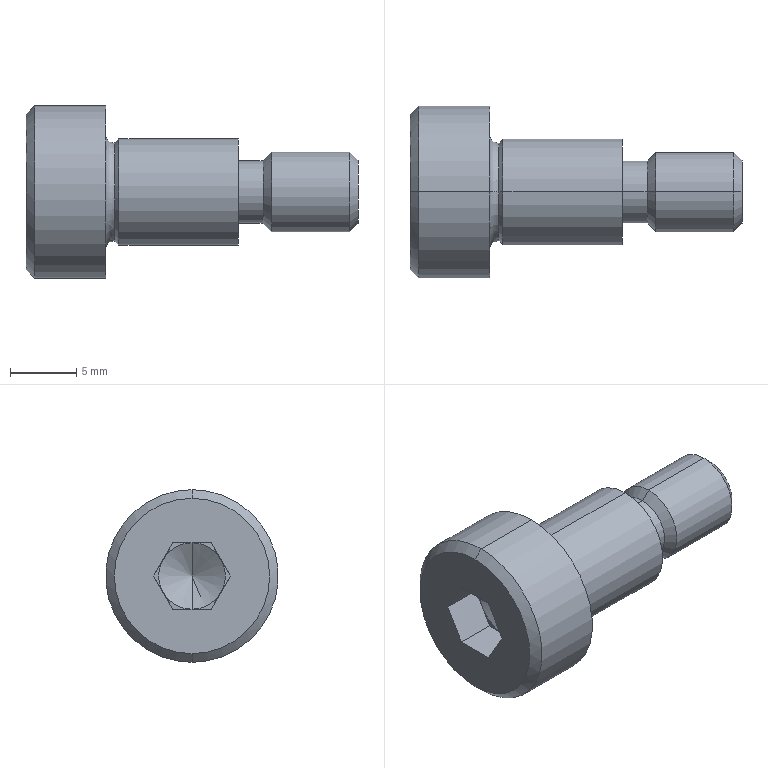Part | STEP file | 11-MSB8_1011_MSB8-10 | 1 solid | 38 faces | box 25 x 13 x 13 mm | volume 1439 mm3 | plane 16 | cone 10 | cylinder 8 | torus 4 | commonest cylinder face diameters 4.7 x2 6 x2 8 x2 13 x2
STEP:
#1=CARTESIAN_POINT('',(0.,0.,4.35));
#2=VERTEX_POINT('',#1);
#3=CARTESIAN_POINT('',(0.6306,0.,3.696));
#4=VERTEX_POINT('',#3);
#5=CARTESIAN_POINT('',(0.6306,0.,4.327));
#6=DIRECTION('',(0.,-1.,0.));
#7=DIRECTION('',(0.,0.,-1.));
#8=AXIS2_PLACEMENT_3D('',#5,#6,#7);
#9=CIRCLE('',#8,0.631);
#10=EDGE_CURVE('',#2,#4,#9,.T.);
#11=ORIENTED_EDGE('',*,*,#10,.T.);
#12=CARTESIAN_POINT('',(0.6306,0.,-3.696));
#13=VERTEX_POINT('',#12);
#14=CARTESIAN_POINT('',(0.6306,0.,0.));
#15=DIRECTION('',(-1.,0.,0.));
#16=DIRECTION('',(0.,0.,1.));
#17=AXIS2_PLACEMENT_3D('',#14,#15,#16);
#18=CIRCLE('',#17,3.696);
#19=EDGE_CURVE('',#4,#13,#18,.T.);
#20=ORIENTED_EDGE('',*,*,#19,.T.);
#21=CARTESIAN_POINT('',(0.,0.,-4.35));
#22=VERTEX_POINT('',#21);
#23=CARTESIAN_POINT('',(0.6306,0.,-4.327));
#24=DIRECTION('',(0.,1.,0.));
#25=DIRECTION('',(0.,0.,1.));
#26=AXIS2_PLACEMENT_3D('',#23,#24,#25);
#27=CIRCLE('',#26,0.631);
#28=EDGE_CURVE('',#22,#13,#27,.T.);
#29=ORIENTED_EDGE('',*,*,#28,.F.);
#30=CARTESIAN_POINT('',(0.,0.,0.));
#31=DIRECTION('',(-1.,0.,0.));
#32=DIRECTION('',(0.,0.,1.));
#33=AXIS2_PLACEMENT_3D('',#30,#31,#32);
#34=CIRCLE('',#33,4.35);
#35=EDGE_CURVE('',#2,#22,#34,.T.);
#36=ORIENTED_EDGE('',*,*,#35,.F.);
#37=EDGE_LOOP('',(#11,#20,#29,#36));
#38=FACE_OUTER_BOUND('',#37,.T.);
#39=CARTESIAN_POINT('',(0.6306,0.,0.));
#40=DIRECTION('',(-1.,0.,0.));
#41=DIRECTION('',(0.,0.,1.));
#42=AXIS2_PLACEMENT_3D('',#39,#40,#41);
#43=TOROIDAL_SURFACE('',#42,4.327,0.631);
#44=ADVANCED_FACE('',(#38),#43,.F.);
#45=ORIENTED_EDGE('',*,*,#28,.T.);
#46=CARTESIAN_POINT('',(0.6306,0.,0.));
#47=DIRECTION('',(-1.,0.,0.));
#48=DIRECTION('',(0.,0.,1.));
#49=AXIS2_PLACEMENT_3D('',#46,#47,#48);
#50=CIRCLE('',#49,3.696);
#51=EDGE_CURVE('',#13,#4,#50,.T.);
#52=ORIENTED_EDGE('',*,*,#51,.T.);
#53=ORIENTED_EDGE('',*,*,#10,.F.);
#54=CARTESIAN_POINT('',(0.,0.,0.));
#55=DIRECTION('',(-1.,0.,0.));
#56=DIRECTION('',(0.,0.,1.));
#57=AXIS2_PLACEMENT_3D('',#54,#55,#56);
#58=CIRCLE('',#57,4.35);
#59=EDGE_CURVE('',#22,#2,#58,.T.);
#60=ORIENTED_EDGE('',*,*,#59,.F.);
#61=EDGE_LOOP('',(#45,#52,#53,#60));
#62=FACE_OUTER_BOUND('',#61,.T.);
#63=CARTESIAN_POINT('',(0.6306,0.,0.));
#64=DIRECTION('',(-1.,0.,0.));
#65=DIRECTION('',(0.,0.,1.));
#66=AXIS2_PLACEMENT_3D('',#63,#64,#65);
#67=TOROIDAL_SURFACE('',#66,4.327,0.631);
#68=ADVANCED_FACE('',(#62),#67,.F.);
#69=CARTESIAN_POINT('',(-1.557,0.,0.));
#70=VERTEX_POINT('',#69);
#71=CARTESIAN_POINT('',(-3.,0.,2.5));
#72=VERTEX_POINT('',#71);
#73=CARTESIAN_POINT('',(-3.,0.,2.5));
#74=DIRECTION('',(-0.5,0.,0.866));
#75=VECTOR('',#74,1000.);
#76=LINE('',#73,#75);
#77=EDGE_CURVE('',#70,#72,#76,.T.);
#78=ORIENTED_EDGE('',*,*,#77,.F.);
#79=CARTESIAN_POINT('',(-3.,0.,-2.5));
#80=VERTEX_POINT('',#79);
#81=CARTESIAN_POINT('',(-3.,0.,-2.5));
#82=DIRECTION('',(-0.5,0.,-0.866));
#83=VECTOR('',#82,1000.);
#84=LINE('',#81,#83);
#85=EDGE_CURVE('',#70,#80,#84,.T.);
#86=ORIENTED_EDGE('',*,*,#85,.T.);
#87=CARTESIAN_POINT('',(-3.,-2.165,-1.25));
#88=VERTEX_POINT('',#87);
#89=CARTESIAN_POINT('',(-3.,0.,0.));
#90=DIRECTION('',(-1.,0.,0.));
#91=DIRECTION('',(0.,0.,1.));
#92=AXIS2_PLACEMENT_3D('',#89,#90,#91);
#93=CIRCLE('',#92,2.5);
#94=EDGE_CURVE('',#80,#88,#93,.T.);
#95=ORIENTED_EDGE('',*,*,#94,.T.);
#96=CARTESIAN_POINT('',(-3.,-2.165,1.25));
#97=VERTEX_POINT('',#96);
#98=CARTESIAN_POINT('',(-3.,0.,0.));
#99=DIRECTION('',(-1.,0.,0.));
#100=DIRECTION('',(0.,0.,1.));
#101=AXIS2_PLACEMENT_3D('',#98,#99,#100);
#102=CIRCLE('',#101,2.5);
#103=EDGE_CURVE('',#88,#97,#102,.T.);
#104=ORIENTED_EDGE('',*,*,#103,.T.);
#105=CARTESIAN_POINT('',(-3.,0.,0.));
#106=DIRECTION('',(-1.,0.,0.));
#107=DIRECTION('',(0.,0.,1.));
#108=AXIS2_PLACEMENT_3D('',#105,#106,#107);
#109=CIRCLE('',#108,2.5);
#110=EDGE_CURVE('',#97,#72,#109,.T.);
#111=ORIENTED_EDGE('',*,*,#110,.T.);
#112=EDGE_LOOP('',(#78,#86,#95,#104,#111));
#113=FACE_OUTER_BOUND('',#112,.T.);
#114=CARTESIAN_POINT('',(-3.,0.,0.));
#115=DIRECTION('',(-1.,0.,0.));
#116=DIRECTION('',(0.,0.,1.));
#117=AXIS2_PLACEMENT_3D('',#114,#115,#116);
#118=CONICAL_SURFACE('',#117,2.5,1.047);
#119=ADVANCED_FACE('',(#113),#118,.F.);
#120=CARTESIAN_POINT('',(-6.,0.,5.85));
#121=VERTEX_POINT('',#120);
#122=CARTESIAN_POINT('',(-6.,0.,-5.85));
#123=VERTEX_POINT('',#122);
#124=CARTESIAN_POINT('',(-6.,0.,0.));
#125=DIRECTION('',(-1.,0.,0.));
#126=DIRECTION('',(0.,0.,1.));
#127=AXIS2_PLACEMENT_3D('',#124,#125,#126);
#128=CIRCLE('',#127,5.85);
#129=EDGE_CURVE('',#121,#123,#128,.T.);
#130=ORIENTED_EDGE('',*,*,#129,.F.);
#131=CARTESIAN_POINT('',(-5.35,0.,6.5));
#132=VERTEX_POINT('',#131);
#133=CARTESIAN_POINT('',(-5.35,0.,6.5));
#134=DIRECTION('',(0.7071,0.,0.7071));
#135=VECTOR('',#134,1000.);
#136=LINE('',#133,#135);
#137=EDGE_CURVE('',#121,#132,#136,.T.);
#138=ORIENTED_EDGE('',*,*,#137,.T.);
#139=CARTESIAN_POINT('',(-5.35,0.,-6.5));
#140=VERTEX_POINT('',#139);
#141=CARTESIAN_POINT('',(-5.35,0.,0.));
#142=DIRECTION('',(-1.,0.,0.));
#143=DIRECTION('',(0.,0.,1.));
#144=AXIS2_PLACEMENT_3D('',#141,#142,#143);
#145=CIRCLE('',#144,6.5);
#146=EDGE_CURVE('',#132,#140,#145,.T.);
#147=ORIENTED_EDGE('',*,*,#146,.T.);
#148=CARTESIAN_POINT('',(-5.35,0.,-6.5));
#149=DIRECTION('',(0.7071,0.,-0.7071));
#150=VECTOR('',#149,1000.);
#151=LINE('',#148,#150);
#152=EDGE_CURVE('',#123,#140,#151,.T.);
#153=ORIENTED_EDGE('',*,*,#152,.F.);
#154=EDGE_LOOP('',(#130,#138,#147,#153));
#155=FACE_OUTER_BOUND('',#154,.T.);
#156=CARTESIAN_POINT('',(-5.35,0.,0.));
#157=DIRECTION('',(1.,0.,0.));
#158=DIRECTION('',(0.,0.,-1.));
#159=AXIS2_PLACEMENT_3D('',#156,#157,#158);
#160=CONICAL_SURFACE('',#159,6.5,0.7854);
#161=ADVANCED_FACE('',(#155),#160,.T.);
#162=CARTESIAN_POINT('',(0.,0.,6.5));
#163=VERTEX_POINT('',#162);
#164=CARTESIAN_POINT('',(0.,0.,-6.5));
#165=VERTEX_POINT('',#164);
#166=CARTESIAN_POINT('',(0.,0.,0.));
#167=DIRECTION('',(-1.,0.,0.));
#168=DIRECTION('',(0.,0.,1.));
#169=AXIS2_PLACEMENT_3D('',#166,#167,#168);
#170=CIRCLE('',#169,6.5);
#171=EDGE_CURVE('',#163,#165,#170,.T.);
#172=ORIENTED_EDGE('',*,*,#171,.T.);
#173=CARTESIAN_POINT('',(19.,0.,-6.5));
#174=DIRECTION('',(-1.,0.,0.));
#175=VECTOR('',#174,1000.);
#176=LINE('',#173,#175);
#177=EDGE_CURVE('',#165,#140,#176,.T.);
#178=ORIENTED_EDGE('',*,*,#177,.T.);
#179=ORIENTED_EDGE('',*,*,#146,.F.);
#180=CARTESIAN_POINT('',(19.,0.,6.5));
#181=DIRECTION('',(-1.,0.,0.));
#182=VECTOR('',#181,1000.);
#183=LINE('',#180,#182);
#184=EDGE_CURVE('',#163,#132,#183,.T.);
#185=ORIENTED_EDGE('',*,*,#184,.F.);
#186=EDGE_LOOP('',(#172,#178,#179,#185));
#187=FACE_OUTER_BOUND('',#186,.T.);
#188=CARTESIAN_POINT('',(19.,0.,0.));
#189=DIRECTION('',(-1.,0.,0.));
#190=DIRECTION('',(0.,0.,1.));
#191=AXIS2_PLACEMENT_3D('',#188,#189,#190);
#192=CYLINDRICAL_SURFACE('',#191,6.5);
#193=ADVANCED_FACE('',(#187),#192,.T.);
#194=ORIENTED_EDGE('',*,*,#51,.F.);
#195=CARTESIAN_POINT('',(0.7,0.,-3.7));
#196=VERTEX_POINT('',#195);
#197=CARTESIAN_POINT('',(0.6306,0.,-4.327));
#198=DIRECTION('',(0.,1.,0.));
#199=DIRECTION('',(0.,0.,1.));
#200=AXIS2_PLACEMENT_3D('',#197,#198,#199);
#201=CIRCLE('',#200,0.631);
#202=EDGE_CURVE('',#13,#196,#201,.T.);
#203=ORIENTED_EDGE('',*,*,#202,.T.);
#204=CARTESIAN_POINT('',(0.7,0.,3.7));
#205=VERTEX_POINT('',#204);
#206=CARTESIAN_POINT('',(0.7,0.,0.));
#207=DIRECTION('',(-1.,0.,0.));
#208=DIRECTION('',(0.,0.,1.));
#209=AXIS2_PLACEMENT_3D('',#206,#207,#208);
#210=CIRCLE('',#209,3.7);
#211=EDGE_CURVE('',#196,#205,#210,.T.);
#212=ORIENTED_EDGE('',*,*,#211,.T.);
#213=CARTESIAN_POINT('',(0.6306,0.,4.327));
#214=DIRECTION('',(0.,-1.,0.));
#215=DIRECTION('',(0.,0.,-1.));
#216=AXIS2_PLACEMENT_3D('',#213,#214,#215);
#217=CIRCLE('',#216,0.631);
#218=EDGE_CURVE('',#4,#205,#217,.T.);
#219=ORIENTED_EDGE('',*,*,#218,.F.);
#220=EDGE_LOOP('',(#194,#203,#212,#219));
#221=FACE_OUTER_BOUND('',#220,.T.);
#222=CARTESIAN_POINT('',(0.6306,0.,0.));
#223=DIRECTION('',(-1.,0.,0.));
#224=DIRECTION('',(0.,0.,1.));
#225=AXIS2_PLACEMENT_3D('',#222,#223,#224);
#226=TOROIDAL_SURFACE('',#225,4.327,0.631);
#227=ADVANCED_FACE('',(#221),#226,.F.);
#228=CARTESIAN_POINT('',(0.7,0.,0.));
#229=DIRECTION('',(-1.,0.,0.));
#230=DIRECTION('',(0.,0.,1.));
#231=AXIS2_PLACEMENT_3D('',#228,#229,#230);
#232=CIRCLE('',#231,3.7);
#233=EDGE_CURVE('',#205,#196,#232,.T.);
#234=ORIENTED_EDGE('',*,*,#233,.F.);
#235=CARTESIAN_POINT('',(1.,0.,4.));
#236=VERTEX_POINT('',#235);
#237=CARTESIAN_POINT('',(1.,0.,4.));
#238=DIRECTION('',(0.7071,0.,0.7071));
#239=VECTOR('',#238,1000.);
#240=LINE('',#237,#239);
#241=EDGE_CURVE('',#205,#236,#240,.T.);
#242=ORIENTED_EDGE('',*,*,#241,.T.);
#243=CARTESIAN_POINT('',(1.,0.,-4.));
#244=VERTEX_POINT('',#243);
#245=CARTESIAN_POINT('',(1.,0.,0.));
#246=DIRECTION('',(-1.,0.,0.));
#247=DIRECTION('',(0.,0.,1.));
#248=AXIS2_PLACEMENT_3D('',#245,#246,#247);
#249=CIRCLE('',#248,4.);
#250=EDGE_CURVE('',#236,#244,#249,.T.);
#251=ORIENTED_EDGE('',*,*,#250,.T.);
#252=CARTESIAN_POINT('',(1.,0.,-4.));
#253=DIRECTION('',(0.7071,0.,-0.7071));
#254=VECTOR('',#253,1000.);
#255=LINE('',#252,#254);
#256=EDGE_CURVE('',#196,#244,#255,.T.);
#257=ORIENTED_EDGE('',*,*,#256,.F.);
#258=EDGE_LOOP('',(#234,#242,#251,#257));
#259=FACE_OUTER_BOUND('',#258,.T.);
#260=CARTESIAN_POINT('',(1.,0.,0.));
#261=DIRECTION('',(1.,0.,0.));
#262=DIRECTION('',(0.,0.,-1.));
#263=AXIS2_PLACEMENT_3D('',#260,#261,#262);
#264=CONICAL_SURFACE('',#263,4.,0.7854);
#265=ADVANCED_FACE('',(#259),#264,.T.);
#266=CARTESIAN_POINT('',(10.,0.,4.));
#267=VERTEX_POINT('',#266);
#268=CARTESIAN_POINT('',(10.,0.,-4.));
#269=VERTEX_POINT('',#268);
#270=CARTESIAN_POINT('',(10.,0.,0.));
#271=DIRECTION('',(-1.,0.,0.));
#272=DIRECTION('',(0.,0.,1.));
#273=AXIS2_PLACEMENT_3D('',#270,#271,#272);
#274=CIRCLE('',#273,4.);
#275=EDGE_CURVE('',#267,#269,#274,.T.);
#276=ORIENTED_EDGE('',*,*,#275,.T.);
#277=CARTESIAN_POINT('',(19.,0.,-4.));
#278=DIRECTION('',(-1.,0.,0.));
#279=VECTOR('',#278,1000.);
#280=LINE('',#277,#279);
#281=EDGE_CURVE('',#269,#244,#280,.T.);
#282=ORIENTED_EDGE('',*,*,#281,.T.);
#283=ORIENTED_EDGE('',*,*,#250,.F.);
#284=CARTESIAN_POINT('',(19.,0.,4.));
#285=DIRECTION('',(-1.,0.,0.));
#286=VECTOR('',#285,1000.);
#287=LINE('',#284,#286);
#288=EDGE_CURVE('',#267,#236,#287,.T.);
#289=ORIENTED_EDGE('',*,*,#288,.F.);
#290=EDGE_LOOP('',(#276,#282,#283,#289));
#291=FACE_OUTER_BOUND('',#290,.T.);
#292=CARTESIAN_POINT('',(19.,0.,0.));
#293=DIRECTION('',(-1.,0.,0.));
#294=DIRECTION('',(0.,0.,1.));
#295=AXIS2_PLACEMENT_3D('',#292,#293,#294);
#296=CYLINDRICAL_SURFACE('',#295,4.);
#297=ADVANCED_FACE('',(#291),#296,.T.);
#298=CARTESIAN_POINT('',(11.85,0.,2.35));
#299=VERTEX_POINT('',#298);
#300=CARTESIAN_POINT('',(11.85,0.,-2.35));
#301=VERTEX_POINT('',#300);
#302=CARTESIAN_POINT('',(11.85,0.,0.));
#303=DIRECTION('',(-1.,0.,0.));
#304=DIRECTION('',(0.,0.,1.));
#305=AXIS2_PLACEMENT_3D('',#302,#303,#304);
#306=CIRCLE('',#305,2.35);
#307=EDGE_CURVE('',#299,#301,#306,.T.);
#308=ORIENTED_EDGE('',*,*,#307,.T.);
#309=CARTESIAN_POINT('',(10.,0.,-2.35));
#310=VERTEX_POINT('',#309);
#311=CARTESIAN_POINT('',(19.,0.,-2.35));
#312=DIRECTION('',(-1.,0.,0.));
#313=VECTOR('',#312,1000.);
#314=LINE('',#311,#313);
#315=EDGE_CURVE('',#301,#310,#314,.T.);
#316=ORIENTED_EDGE('',*,*,#315,.T.);
#317=CARTESIAN_POINT('',(10.,0.,2.35));
#318=VERTEX_POINT('',#317);
#319=CARTESIAN_POINT('',(10.,0.,0.));
#320=DIRECTION('',(-1.,0.,0.));
#321=DIRECTION('',(0.,0.,1.));
#322=AXIS2_PLACEMENT_3D('',#319,#320,#321);
#323=CIRCLE('',#322,2.35);
#324=EDGE_CURVE('',#318,#310,#323,.T.);
#325=ORIENTED_EDGE('',*,*,#324,.F.);
#326=CARTESIAN_POINT('',(19.,0.,2.35));
#327=DIRECTION('',(-1.,0.,0.));
#328=VECTOR('',#327,1000.);
#329=LINE('',#326,#328);
#330=EDGE_CURVE('',#299,#318,#329,.T.);
#331=ORIENTED_EDGE('',*,*,#330,.F.);
#332=EDGE_LOOP('',(#308,#316,#325,#331));
#333=FACE_OUTER_BOUND('',#332,.T.);
#334=CARTESIAN_POINT('',(19.,0.,0.));
#335=DIRECTION('',(-1.,0.,0.));
#336=DIRECTION('',(0.,0.,1.));
#337=AXIS2_PLACEMENT_3D('',#334,#335,#336);
#338=CYLINDRICAL_SURFACE('',#337,2.35);
#339=ADVANCED_FACE('',(#333),#338,.T.);
#340=ORIENTED_EDGE('',*,*,#307,.F.);
#341=CARTESIAN_POINT('',(12.5,0.,3.));
#342=VERTEX_POINT('',#341);
#343=CARTESIAN_POINT('',(12.5,0.,3.));
#344=DIRECTION('',(0.7071,0.,0.7071));
#345=VECTOR('',#344,1000.);
#346=LINE('',#343,#345);
#347=EDGE_CURVE('',#299,#342,#346,.T.);
#348=ORIENTED_EDGE('',*,*,#347,.T.);
#349=CARTESIAN_POINT('',(12.5,0.,-3.));
#350=VERTEX_POINT('',#349);
#351=CARTESIAN_POINT('',(12.5,0.,0.));
#352=DIRECTION('',(-1.,0.,0.));
#353=DIRECTION('',(0.,0.,1.));
#354=AXIS2_PLACEMENT_3D('',#351,#352,#353);
#355=CIRCLE('',#354,3.);
#356=EDGE_CURVE('',#342,#350,#355,.T.);
#357=ORIENTED_EDGE('',*,*,#356,.T.);
#358=CARTESIAN_POINT('',(12.5,0.,-3.));
#359=DIRECTION('',(0.7071,0.,-0.7071));
#360=VECTOR('',#359,1000.);
#361=LINE('',#358,#360);
#362=EDGE_CURVE('',#301,#350,#361,.T.);
#363=ORIENTED_EDGE('',*,*,#362,.F.);
#364=EDGE_LOOP('',(#340,#348,#357,#363));
#365=FACE_OUTER_BOUND('',#364,.T.);
#366=CARTESIAN_POINT('',(12.5,0.,0.));
#367=DIRECTION('',(1.,0.,0.));
#368=DIRECTION('',(0.,0.,-1.));
#369=AXIS2_PLACEMENT_3D('',#366,#367,#368);
#370=CONICAL_SURFACE('',#369,3.,0.7854);
#371=ADVANCED_FACE('',(#365),#370,.T.);
#372=CARTESIAN_POINT('',(18.387,0.,3.));
#373=VERTEX_POINT('',#372);
#374=CARTESIAN_POINT('',(18.387,0.,-3.));
#375=VERTEX_POINT('',#374);
#376=CARTESIAN_POINT('',(18.387,0.,0.));
#377=DIRECTION('',(-1.,0.,0.));
#378=DIRECTION('',(0.,0.,1.));
#379=AXIS2_PLACEMENT_3D('',#376,#377,#378);
#380=CIRCLE('',#379,3.);
#381=EDGE_CURVE('',#373,#375,#380,.T.);
#382=ORIENTED_EDGE('',*,*,#381,.T.);
#383=CARTESIAN_POINT('',(19.,0.,-3.));
#384=DIRECTION('',(-1.,0.,0.));
#385=VECTOR('',#384,1000.);
#386=LINE('',#383,#385);
#387=EDGE_CURVE('',#375,#350,#386,.T.);
#388=ORIENTED_EDGE('',*,*,#387,.T.);
#389=ORIENTED_EDGE('',*,*,#356,.F.);
#390=CARTESIAN_POINT('',(19.,0.,3.));
#391=DIRECTION('',(-1.,0.,0.));
#392=VECTOR('',#391,1000.);
#393=LINE('',#390,#392);
#394=EDGE_CURVE('',#373,#342,#393,.T.);
#395=ORIENTED_EDGE('',*,*,#394,.F.);
#396=EDGE_LOOP('',(#382,#388,#389,#395));
#397=FACE_OUTER_BOUND('',#396,.T.);
#398=CARTESIAN_POINT('',(19.,0.,0.));
#399=DIRECTION('',(-1.,0.,0.));
#400=DIRECTION('',(0.,0.,1.));
#401=AXIS2_PLACEMENT_3D('',#398,#399,#400);
#402=CYLINDRICAL_SURFACE('',#401,3.);
#403=ADVANCED_FACE('',(#397),#402,.T.);
#404=CARTESIAN_POINT('',(19.,0.,2.386));
#405=VERTEX_POINT('',#404);
#406=CARTESIAN_POINT('',(19.,0.,-2.386));
#407=VERTEX_POINT('',#406);
#408=CARTESIAN_POINT('',(19.,0.,0.));
#409=DIRECTION('',(-1.,0.,0.));
#410=DIRECTION('',(0.,0.,1.));
#411=AXIS2_PLACEMENT_3D('',#408,#409,#410);
#412=CIRCLE('',#411,2.386);
#413=EDGE_CURVE('',#405,#407,#412,.T.);
#414=ORIENTED_EDGE('',*,*,#413,.T.);
#415=CARTESIAN_POINT('',(19.,0.,-2.386));
#416=DIRECTION('',(-0.7071,0.,-0.7071));
#417=VECTOR('',#416,1000.);
#418=LINE('',#415,#417);
#419=EDGE_CURVE('',#407,#375,#418,.T.);
#420=ORIENTED_EDGE('',*,*,#419,.T.);
#421=ORIENTED_EDGE('',*,*,#381,.F.);
#422=CARTESIAN_POINT('',(19.,0.,2.386));
#423=DIRECTION('',(-0.7071,0.,0.7071));
#424=VECTOR('',#423,1000.);
#425=LINE('',#422,#424);
#426=EDGE_CURVE('',#405,#373,#425,.T.);
#427=ORIENTED_EDGE('',*,*,#426,.F.);
#428=EDGE_LOOP('',(#414,#420,#421,#427));
#429=FACE_OUTER_BOUND('',#428,.T.);
#430=CARTESIAN_POINT('',(19.,0.,0.));
#431=DIRECTION('',(-1.,0.,0.));
#432=DIRECTION('',(0.,0.,1.));
#433=AXIS2_PLACEMENT_3D('',#430,#431,#432);
#434=CONICAL_SURFACE('',#433,2.386,0.7854);
#435=ADVANCED_FACE('',(#429),#434,.T.);
#436=CARTESIAN_POINT('',(-6.,0.,0.));
#437=DIRECTION('',(-1.,0.,0.));
#438=DIRECTION('',(0.,0.,1.));
#439=AXIS2_PLACEMENT_3D('',#436,#437,#438);
#440=CIRCLE('',#439,5.85);
#441=EDGE_CURVE('',#123,#121,#440,.T.);
#442=ORIENTED_EDGE('',*,*,#441,.T.);
#443=ORIENTED_EDGE('',*,*,#129,.T.);
#444=EDGE_LOOP('',(#442,#443));
#445=FACE_OUTER_BOUND('',#444,.T.);
#446=CARTESIAN_POINT('',(-6.,-1.443,2.5));
#447=VERTEX_POINT('',#446);
#448=CARTESIAN_POINT('',(-6.,-2.887,0.));
#449=VERTEX_POINT('',#448);
#450=CARTESIAN_POINT('',(-6.,-1.443,2.5));
#451=DIRECTION('',(0.,-0.5,-0.866));
#452=VECTOR('',#451,1000.);
#453=LINE('',#450,#452);
#454=EDGE_CURVE('',#447,#449,#453,.T.);
#455=ORIENTED_EDGE('',*,*,#454,.T.);
#456=CARTESIAN_POINT('',(-6.,-1.443,-2.5));
#457=VERTEX_POINT('',#456);
#458=CARTESIAN_POINT('',(-6.,-2.887,0.));
#459=DIRECTION('',(0.,0.5,-0.866));
#460=VECTOR('',#459,1000.);
#461=LINE('',#458,#460);
#462=EDGE_CURVE('',#449,#457,#461,.T.);
#463=ORIENTED_EDGE('',*,*,#462,.T.);
#464=CARTESIAN_POINT('',(-6.,1.443,-2.5));
#465=VERTEX_POINT('',#464);
#466=CARTESIAN_POINT('',(-6.,-1.443,-2.5));
#467=DIRECTION('',(0.,1.,0.));
#468=VECTOR('',#467,1000.);
#469=LINE('',#466,#468);
#470=EDGE_CURVE('',#457,#465,#469,.T.);
#471=ORIENTED_EDGE('',*,*,#470,.T.);
#472=CARTESIAN_POINT('',(-6.,2.887,0.));
#473=VERTEX_POINT('',#472);
#474=CARTESIAN_POINT('',(-6.,1.443,-2.5));
#475=DIRECTION('',(0.,0.5,0.866));
#476=VECTOR('',#475,1000.);
#477=LINE('',#474,#476);
#478=EDGE_CURVE('',#465,#473,#477,.T.);
#479=ORIENTED_EDGE('',*,*,#478,.T.);
#480=CARTESIAN_POINT('',(-6.,1.443,2.5));
#481=VERTEX_POINT('',#480);
#482=CARTESIAN_POINT('',(-6.,2.887,0.));
#483=DIRECTION('',(0.,-0.5,0.866));
#484=VECTOR('',#483,1000.);
#485=LINE('',#482,#484);
#486=EDGE_CURVE('',#473,#481,#485,.T.);
#487=ORIENTED_EDGE('',*,*,#486,.T.);
#488=CARTESIAN_POINT('',(-6.,1.443,2.5));
#489=DIRECTION('',(0.,-1.,0.));
#490=VECTOR('',#489,1000.);
#491=LINE('',#488,#490);
#492=EDGE_CURVE('',#481,#447,#491,.T.);
#493=ORIENTED_EDGE('',*,*,#492,.T.);
#494=EDGE_LOOP('',(#455,#463,#471,#479,#487,#493));
#495=FACE_BOUND('',#494,.T.);
#496=CARTESIAN_POINT('',(-6.,2.5,0.));
#497=DIRECTION('',(1.,0.,0.));
#498=DIRECTION('',(0.,0.,-1.));
#499=AXIS2_PLACEMENT_3D('',#496,#497,#498);
#500=PLANE('',#499);
#501=ADVANCED_FACE('',(#445,#495),#500,.F.);
#502=ORIENTED_EDGE('',*,*,#413,.F.);
#503=CARTESIAN_POINT('',(19.,0.,0.));
#504=DIRECTION('',(-1.,0.,0.));
#505=DIRECTION('',(0.,0.,1.));
#506=AXIS2_PLACEMENT_3D('',#503,#504,#505);
#507=CIRCLE('',#506,2.386);
#508=EDGE_CURVE('',#407,#405,#507,.T.);
#509=ORIENTED_EDGE('',*,*,#508,.F.);
#510=EDGE_LOOP('',(#502,#509));
#511=FACE_OUTER_BOUND('',#510,.T.);
#512=CARTESIAN_POINT('',(19.,2.386,0.));
#513=DIRECTION('',(-1.,0.,0.));
#514=DIRECTION('',(0.,0.,1.));
#515=AXIS2_PLACEMENT_3D('',#512,#513,#514);
#516=PLANE('',#515);
#517=ADVANCED_FACE('',(#511),#516,.F.);
#518=ORIENTED_EDGE('',*,*,#419,.F.);
#519=ORIENTED_EDGE('',*,*,#508,.T.);
#520=ORIENTED_EDGE('',*,*,#426,.T.);
#521=CARTESIAN_POINT('',(18.387,0.,0.));
#522=DIRECTION('',(-1.,0.,0.));
#523=DIRECTION('',(0.,0.,1.));
#524=AXIS2_PLACEMENT_3D('',#521,#522,#523);
#525=CIRCLE('',#524,3.);
#526=EDGE_CURVE('',#375,#373,#525,.T.);
#527=ORIENTED_EDGE('',*,*,#526,.F.);
#528=EDGE_LOOP('',(#518,#519,#520,#527));
#529=FACE_OUTER_BOUND('',#528,.T.);
#530=CARTESIAN_POINT('',(19.,0.,0.));
#531=DIRECTION('',(-1.,0.,0.));
#532=DIRECTION('',(0.,0.,1.));
#533=AXIS2_PLACEMENT_3D('',#530,#531,#532);
#534=CONICAL_SURFACE('',#533,2.386,0.7854);
#535=ADVANCED_FACE('',(#529),#534,.T.);
#536=ORIENTED_EDGE('',*,*,#387,.F.);
#537=ORIENTED_EDGE('',*,*,#526,.T.);
#538=ORIENTED_EDGE('',*,*,#394,.T.);
#539=CARTESIAN_POINT('',(12.5,0.,0.));
#540=DIRECTION('',(-1.,0.,0.));
#541=DIRECTION('',(0.,0.,1.));
#542=AXIS2_PLACEMENT_3D('',#539,#540,#541);
#543=CIRCLE('',#542,3.);
#544=EDGE_CURVE('',#350,#342,#543,.T.);
#545=ORIENTED_EDGE('',*,*,#544,.F.);
#546=EDGE_LOOP('',(#536,#537,#538,#545));
#547=FACE_OUTER_BOUND('',#546,.T.);
#548=CARTESIAN_POINT('',(19.,0.,0.));
#549=DIRECTION('',(-1.,0.,0.));
#550=DIRECTION('',(0.,0.,1.));
#551=AXIS2_PLACEMENT_3D('',#548,#549,#550);
#552=CYLINDRICAL_SURFACE('',#551,3.);
#553=ADVANCED_FACE('',(#547),#552,.T.);
#554=ORIENTED_EDGE('',*,*,#347,.F.);
#555=CARTESIAN_POINT('',(11.85,0.,0.));
#556=DIRECTION('',(-1.,0.,0.));
#557=DIRECTION('',(0.,0.,1.));
#558=AXIS2_PLACEMENT_3D('',#555,#556,#557);
#559=CIRCLE('',#558,2.35);
#560=EDGE_CURVE('',#301,#299,#559,.T.);
#561=ORIENTED_EDGE('',*,*,#560,.F.);
#562=ORIENTED_EDGE('',*,*,#362,.T.);
#563=ORIENTED_EDGE('',*,*,#544,.T.);
#564=EDGE_LOOP('',(#554,#561,#562,#563));
#565=FACE_OUTER_BOUND('',#564,.T.);
#566=CARTESIAN_POINT('',(12.5,0.,0.));
#567=DIRECTION('',(1.,0.,0.));
#568=DIRECTION('',(0.,0.,-1.));
#569=AXIS2_PLACEMENT_3D('',#566,#567,#568);
#570=CONICAL_SURFACE('',#569,3.,0.7854);
#571=ADVANCED_FACE('',(#565),#570,.T.);
#572=ORIENTED_EDGE('',*,*,#315,.F.);
#573=ORIENTED_EDGE('',*,*,#560,.T.);
#574=ORIENTED_EDGE('',*,*,#330,.T.);
#575=CARTESIAN_POINT('',(10.,0.,0.));
#576=DIRECTION('',(-1.,0.,0.));
#577=DIRECTION('',(0.,0.,1.));
#578=AXIS2_PLACEMENT_3D('',#575,#576,#577);
#579=CIRCLE('',#578,2.35);
#580=EDGE_CURVE('',#310,#318,#579,.T.);
#581=ORIENTED_EDGE('',*,*,#580,.F.);
#582=EDGE_LOOP('',(#572,#573,#574,#581));
#583=FACE_OUTER_BOUND('',#582,.T.);
#584=CARTESIAN_POINT('',(19.,0.,0.));
#585=DIRECTION('',(-1.,0.,0.));
#586=DIRECTION('',(0.,0.,1.));
#587=AXIS2_PLACEMENT_3D('',#584,#585,#586);
#588=CYLINDRICAL_SURFACE('',#587,2.35);
#589=ADVANCED_FACE('',(#583),#588,.T.);
#590=ORIENTED_EDGE('',*,*,#275,.F.);
#591=CARTESIAN_POINT('',(10.,0.,0.));
#592=DIRECTION('',(-1.,0.,0.));
#593=DIRECTION('',(0.,0.,1.));
#594=AXIS2_PLACEMENT_3D('',#591,#592,#593);
#595=CIRCLE('',#594,4.);
#596=EDGE_CURVE('',#269,#267,#595,.T.);
#597=ORIENTED_EDGE('',*,*,#596,.F.);
#598=EDGE_LOOP('',(#590,#597));
#599=FACE_OUTER_BOUND('',#598,.T.);
#600=ORIENTED_EDGE('',*,*,#324,.T.);
#601=ORIENTED_EDGE('',*,*,#580,.T.);
#602=EDGE_LOOP('',(#600,#601));
#603=FACE_BOUND('',#602,.T.);
#604=CARTESIAN_POINT('',(10.,4.,0.));
#605=DIRECTION('',(-1.,0.,0.));
#606=DIRECTION('',(0.,0.,1.));
#607=AXIS2_PLACEMENT_3D('',#604,#605,#606);
#608=PLANE('',#607);
#609=ADVANCED_FACE('',(#599,#603),#608,.F.);
#610=ORIENTED_EDGE('',*,*,#281,.F.);
#611=ORIENTED_EDGE('',*,*,#596,.T.);
#612=ORIENTED_EDGE('',*,*,#288,.T.);
#613=CARTESIAN_POINT('',(1.,0.,0.));
#614=DIRECTION('',(-1.,0.,0.));
#615=DIRECTION('',(0.,0.,1.));
#616=AXIS2_PLACEMENT_3D('',#613,#614,#615);
#617=CIRCLE('',#616,4.);
#618=EDGE_CURVE('',#244,#236,#617,.T.);
#619=ORIENTED_EDGE('',*,*,#618,.F.);
#620=EDGE_LOOP('',(#610,#611,#612,#619));
#621=FACE_OUTER_BOUND('',#620,.T.);
#622=CARTESIAN_POINT('',(19.,0.,0.));
#623=DIRECTION('',(-1.,0.,0.));
#624=DIRECTION('',(0.,0.,1.));
#625=AXIS2_PLACEMENT_3D('',#622,#623,#624);
#626=CYLINDRICAL_SURFACE('',#625,4.);
#627=ADVANCED_FACE('',(#621),#626,.T.);
#628=ORIENTED_EDGE('',*,*,#241,.F.);
#629=ORIENTED_EDGE('',*,*,#211,.F.);
#630=ORIENTED_EDGE('',*,*,#256,.T.);
#631=ORIENTED_EDGE('',*,*,#618,.T.);
#632=EDGE_LOOP('',(#628,#629,#630,#631));
#633=FACE_OUTER_BOUND('',#632,.T.);
#634=CARTESIAN_POINT('',(1.,0.,0.));
#635=DIRECTION('',(1.,0.,0.));
#636=DIRECTION('',(0.,0.,-1.));
#637=AXIS2_PLACEMENT_3D('',#634,#635,#636);
#638=CONICAL_SURFACE('',#637,4.,0.7854);
#639=ADVANCED_FACE('',(#633),#638,.T.);
#640=ORIENTED_EDGE('',*,*,#19,.F.);
#641=ORIENTED_EDGE('',*,*,#218,.T.);
#642=ORIENTED_EDGE('',*,*,#233,.T.);
#643=ORIENTED_EDGE('',*,*,#202,.F.);
#644=EDGE_LOOP('',(#640,#641,#642,#643));
#645=FACE_OUTER_BOUND('',#644,.T.);
#646=CARTESIAN_POINT('',(0.6306,0.,0.));
#647=DIRECTION('',(-1.,0.,0.));
#648=DIRECTION('',(0.,0.,1.));
#649=AXIS2_PLACEMENT_3D('',#646,#647,#648);
#650=TOROIDAL_SURFACE('',#649,4.327,0.631);
#651=ADVANCED_FACE('',(#645),#650,.F.);
#652=ORIENTED_EDGE('',*,*,#171,.F.);
#653=CARTESIAN_POINT('',(0.,0.,0.));
#654=DIRECTION('',(-1.,0.,0.));
#655=DIRECTION('',(0.,0.,1.));
#656=AXIS2_PLACEMENT_3D('',#653,#654,#655);
#657=CIRCLE('',#656,6.5);
#658=EDGE_CURVE('',#165,#163,#657,.T.);
#659=ORIENTED_EDGE('',*,*,#658,.F.);
#660=EDGE_LOOP('',(#652,#659));
#661=FACE_OUTER_BOUND('',#660,.T.);
#662=ORIENTED_EDGE('',*,*,#35,.T.);
#663=ORIENTED_EDGE('',*,*,#59,.T.);
#664=EDGE_LOOP('',(#662,#663));
#665=FACE_BOUND('',#664,.T.);
#666=CARTESIAN_POINT('',(0.,6.5,0.));
#667=DIRECTION('',(-1.,0.,0.));
#668=DIRECTION('',(0.,0.,1.));
#669=AXIS2_PLACEMENT_3D('',#666,#667,#668);
#670=PLANE('',#669);
#671=ADVANCED_FACE('',(#661,#665),#670,.F.);
#672=ORIENTED_EDGE('',*,*,#177,.F.);
#673=ORIENTED_EDGE('',*,*,#658,.T.);
#674=ORIENTED_EDGE('',*,*,#184,.T.);
#675=CARTESIAN_POINT('',(-5.35,0.,0.));
#676=DIRECTION('',(-1.,0.,0.));
#677=DIRECTION('',(0.,0.,1.));
#678=AXIS2_PLACEMENT_3D('',#675,#676,#677);
#679=CIRCLE('',#678,6.5);
#680=EDGE_CURVE('',#140,#132,#679,.T.);
#681=ORIENTED_EDGE('',*,*,#680,.F.);
#682=EDGE_LOOP('',(#672,#673,#674,#681));
#683=FACE_OUTER_BOUND('',#682,.T.);
#684=CARTESIAN_POINT('',(19.,0.,0.));
#685=DIRECTION('',(-1.,0.,0.));
#686=DIRECTION('',(0.,0.,1.));
#687=AXIS2_PLACEMENT_3D('',#684,#685,#686);
#688=CYLINDRICAL_SURFACE('',#687,6.5);
#689=ADVANCED_FACE('',(#683),#688,.T.);
#690=ORIENTED_EDGE('',*,*,#137,.F.);
#691=ORIENTED_EDGE('',*,*,#441,.F.);
#692=ORIENTED_EDGE('',*,*,#152,.T.);
#693=ORIENTED_EDGE('',*,*,#680,.T.);
#694=EDGE_LOOP('',(#690,#691,#692,#693));
#695=FACE_OUTER_BOUND('',#694,.T.);
#696=CARTESIAN_POINT('',(-5.35,0.,0.));
#697=DIRECTION('',(1.,0.,0.));
#698=DIRECTION('',(0.,0.,-1.));
#699=AXIS2_PLACEMENT_3D('',#696,#697,#698);
#700=CONICAL_SURFACE('',#699,6.5,0.7854);
#701=ADVANCED_FACE('',(#695),#700,.T.);
#702=ORIENTED_EDGE('',*,*,#486,.F.);
#703=CARTESIAN_POINT('',(-3.,2.887,0.));
#704=VERTEX_POINT('',#703);
#705=CARTESIAN_POINT('',(-3.,2.887,0.));
#706=DIRECTION('',(-1.,0.,0.));
#707=VECTOR('',#706,1000.);
#708=LINE('',#705,#707);
#709=EDGE_CURVE('',#704,#473,#708,.T.);
#710=ORIENTED_EDGE('',*,*,#709,.F.);
#711=CARTESIAN_POINT('',(-3.,2.165,1.25));
#712=VERTEX_POINT('',#711);
#713=CARTESIAN_POINT('',(-3.,2.887,0.));
#714=DIRECTION('',(0.,-0.5,0.866));
#715=VECTOR('',#714,1000.);
#716=LINE('',#713,#715);
#717=EDGE_CURVE('',#704,#712,#716,.T.);
#718=ORIENTED_EDGE('',*,*,#717,.T.);
#719=CARTESIAN_POINT('',(-3.,1.443,2.5));
#720=VERTEX_POINT('',#719);
#721=CARTESIAN_POINT('',(-3.,2.887,0.));
#722=DIRECTION('',(0.,-0.5,0.866));
#723=VECTOR('',#722,1000.);
#724=LINE('',#721,#723);
#725=EDGE_CURVE('',#712,#720,#724,.T.);
#726=ORIENTED_EDGE('',*,*,#725,.T.);
#727=CARTESIAN_POINT('',(-3.,1.443,2.5));
#728=DIRECTION('',(-1.,0.,0.));
#729=VECTOR('',#728,1000.);
#730=LINE('',#727,#729);
#731=EDGE_CURVE('',#720,#481,#730,.T.);
#732=ORIENTED_EDGE('',*,*,#731,.T.);
#733=EDGE_LOOP('',(#702,#710,#718,#726,#732));
#734=FACE_OUTER_BOUND('',#733,.T.);
#735=CARTESIAN_POINT('',(-3.,2.887,0.));
#736=DIRECTION('',(0.,-0.866,-0.5));
#737=DIRECTION('',(0.,0.5,-0.866));
#738=AXIS2_PLACEMENT_3D('',#735,#736,#737);
#739=PLANE('',#738);
#740=ADVANCED_FACE('',(#734),#739,.T.);
#741=ORIENTED_EDGE('',*,*,#492,.F.);
#742=ORIENTED_EDGE('',*,*,#731,.F.);
#743=CARTESIAN_POINT('',(-3.,1.443,2.5));
#744=DIRECTION('',(0.,-1.,0.));
#745=VECTOR('',#744,1000.);
#746=LINE('',#743,#745);
#747=EDGE_CURVE('',#720,#72,#746,.T.);
#748=ORIENTED_EDGE('',*,*,#747,.T.);
#749=CARTESIAN_POINT('',(-3.,-1.443,2.5));
#750=VERTEX_POINT('',#749);
#751=CARTESIAN_POINT('',(-3.,1.443,2.5));
#752=DIRECTION('',(0.,-1.,0.));
#753=VECTOR('',#752,1000.);
#754=LINE('',#751,#753);
#755=EDGE_CURVE('',#72,#750,#754,.T.);
#756=ORIENTED_EDGE('',*,*,#755,.T.);
#757=CARTESIAN_POINT('',(-3.,-1.443,2.5));
#758=DIRECTION('',(-1.,0.,0.));
#759=VECTOR('',#758,1000.);
#760=LINE('',#757,#759);
#761=EDGE_CURVE('',#750,#447,#760,.T.);
#762=ORIENTED_EDGE('',*,*,#761,.T.);
#763=EDGE_LOOP('',(#741,#742,#748,#756,#762));
#764=FACE_OUTER_BOUND('',#763,.T.);
#765=CARTESIAN_POINT('',(-3.,1.443,2.5));
#766=DIRECTION('',(0.,0.,-1.));
#767=DIRECTION('',(-1.,0.,0.));
#768=AXIS2_PLACEMENT_3D('',#765,#766,#767);
#769=PLANE('',#768);
#770=ADVANCED_FACE('',(#764),#769,.T.);
#771=ORIENTED_EDGE('',*,*,#454,.F.);
#772=ORIENTED_EDGE('',*,*,#761,.F.);
#773=CARTESIAN_POINT('',(-3.,-1.443,2.5));
#774=DIRECTION('',(0.,-0.5,-0.866));
#775=VECTOR('',#774,1000.);
#776=LINE('',#773,#775);
#777=EDGE_CURVE('',#750,#97,#776,.T.);
#778=ORIENTED_EDGE('',*,*,#777,.T.);
#779=CARTESIAN_POINT('',(-3.,-2.887,0.));
#780=VERTEX_POINT('',#779);
#781=CARTESIAN_POINT('',(-3.,-1.443,2.5));
#782=DIRECTION('',(0.,-0.5,-0.866));
#783=VECTOR('',#782,1000.);
#784=LINE('',#781,#783);
#785=EDGE_CURVE('',#97,#780,#784,.T.);
#786=ORIENTED_EDGE('',*,*,#785,.T.);
#787=CARTESIAN_POINT('',(-3.,-2.887,0.));
#788=DIRECTION('',(-1.,0.,0.));
#789=VECTOR('',#788,1000.);
#790=LINE('',#787,#789);
#791=EDGE_CURVE('',#780,#449,#790,.T.);
#792=ORIENTED_EDGE('',*,*,#791,.T.);
#793=EDGE_LOOP('',(#771,#772,#778,#786,#792));
#794=FACE_OUTER_BOUND('',#793,.T.);
#795=CARTESIAN_POINT('',(-3.,-1.443,2.5));
#796=DIRECTION('',(0.,0.866,-0.5));
#797=DIRECTION('',(0.,0.5,0.866));
#798=AXIS2_PLACEMENT_3D('',#795,#796,#797);
#799=PLANE('',#798);
#800=ADVANCED_FACE('',(#794),#799,.T.);
#801=ORIENTED_EDGE('',*,*,#462,.F.);
#802=ORIENTED_EDGE('',*,*,#791,.F.);
#803=CARTESIAN_POINT('',(-3.,-2.887,0.));
#804=DIRECTION('',(0.,0.5,-0.866));
#805=VECTOR('',#804,1000.);
#806=LINE('',#803,#805);
#807=EDGE_CURVE('',#780,#88,#806,.T.);
#808=ORIENTED_EDGE('',*,*,#807,.T.);
#809=CARTESIAN_POINT('',(-3.,-1.443,-2.5));
#810=VERTEX_POINT('',#809);
#811=CARTESIAN_POINT('',(-3.,-2.887,0.));
#812=DIRECTION('',(0.,0.5,-0.866));
#813=VECTOR('',#812,1000.);
#814=LINE('',#811,#813);
#815=EDGE_CURVE('',#88,#810,#814,.T.);
#816=ORIENTED_EDGE('',*,*,#815,.T.);
#817=CARTESIAN_POINT('',(-3.,-1.443,-2.5));
#818=DIRECTION('',(-1.,0.,0.));
#819=VECTOR('',#818,1000.);
#820=LINE('',#817,#819);
#821=EDGE_CURVE('',#810,#457,#820,.T.);
#822=ORIENTED_EDGE('',*,*,#821,.T.);
#823=EDGE_LOOP('',(#801,#802,#808,#816,#822));
#824=FACE_OUTER_BOUND('',#823,.T.);
#825=CARTESIAN_POINT('',(-3.,-2.887,0.));
#826=DIRECTION('',(0.,0.866,0.5));
#827=DIRECTION('',(0.,-0.5,0.866));
#828=AXIS2_PLACEMENT_3D('',#825,#826,#827);
#829=PLANE('',#828);
#830=ADVANCED_FACE('',(#824),#829,.T.);
#831=ORIENTED_EDGE('',*,*,#470,.F.);
#832=ORIENTED_EDGE('',*,*,#821,.F.);
#833=CARTESIAN_POINT('',(-3.,-1.443,-2.5));
#834=DIRECTION('',(0.,1.,0.));
#835=VECTOR('',#834,1000.);
#836=LINE('',#833,#835);
#837=EDGE_CURVE('',#810,#80,#836,.T.);
#838=ORIENTED_EDGE('',*,*,#837,.T.);
#839=CARTESIAN_POINT('',(-3.,1.443,-2.5));
#840=VERTEX_POINT('',#839);
#841=CARTESIAN_POINT('',(-3.,-1.443,-2.5));
#842=DIRECTION('',(0.,1.,0.));
#843=VECTOR('',#842,1000.);
#844=LINE('',#841,#843);
#845=EDGE_CURVE('',#80,#840,#844,.T.);
#846=ORIENTED_EDGE('',*,*,#845,.T.);
#847=CARTESIAN_POINT('',(-3.,1.443,-2.5));
#848=DIRECTION('',(-1.,0.,0.));
#849=VECTOR('',#848,1000.);
#850=LINE('',#847,#849);
#851=EDGE_CURVE('',#840,#465,#850,.T.);
#852=ORIENTED_EDGE('',*,*,#851,.T.);
#853=EDGE_LOOP('',(#831,#832,#838,#846,#852));
#854=FACE_OUTER_BOUND('',#853,.T.);
#855=CARTESIAN_POINT('',(-3.,-1.443,-2.5));
#856=DIRECTION('',(0.,0.,1.));
#857=DIRECTION('',(1.,0.,0.));
#858=AXIS2_PLACEMENT_3D('',#855,#856,#857);
#859=PLANE('',#858);
#860=ADVANCED_FACE('',(#854),#859,.T.);
#861=ORIENTED_EDGE('',*,*,#478,.F.);
#862=ORIENTED_EDGE('',*,*,#851,.F.);
#863=CARTESIAN_POINT('',(-3.,2.165,-1.25));
#864=VERTEX_POINT('',#863);
#865=CARTESIAN_POINT('',(-3.,1.443,-2.5));
#866=DIRECTION('',(0.,0.5,0.866));
#867=VECTOR('',#866,1000.);
#868=LINE('',#865,#867);
#869=EDGE_CURVE('',#840,#864,#868,.T.);
#870=ORIENTED_EDGE('',*,*,#869,.T.);
#871=CARTESIAN_POINT('',(-3.,1.443,-2.5));
#872=DIRECTION('',(0.,0.5,0.866));
#873=VECTOR('',#872,1000.);
#874=LINE('',#871,#873);
#875=EDGE_CURVE('',#864,#704,#874,.T.);
#876=ORIENTED_EDGE('',*,*,#875,.T.);
#877=ORIENTED_EDGE('',*,*,#709,.T.);
#878=EDGE_LOOP('',(#861,#862,#870,#876,#877));
#879=FACE_OUTER_BOUND('',#878,.T.);
#880=CARTESIAN_POINT('',(-3.,1.443,-2.5));
#881=DIRECTION('',(0.,-0.866,0.5));
#882=DIRECTION('',(0.,-0.5,-0.866));
#883=AXIS2_PLACEMENT_3D('',#880,#881,#882);
#884=PLANE('',#883);
#885=ADVANCED_FACE('',(#879),#884,.T.);
#886=ORIENTED_EDGE('',*,*,#837,.F.);
#887=ORIENTED_EDGE('',*,*,#815,.F.);
#888=ORIENTED_EDGE('',*,*,#94,.F.);
#889=EDGE_LOOP('',(#886,#887,#888));
#890=FACE_OUTER_BOUND('',#889,.T.);
#891=CARTESIAN_POINT('',(-3.,0.,0.));
#892=DIRECTION('',(1.,0.,0.));
#893=DIRECTION('',(0.,0.,-1.));
#894=AXIS2_PLACEMENT_3D('',#891,#892,#893);
#895=PLANE('',#894);
#896=ADVANCED_FACE('',(#890),#895,.F.);
#897=ORIENTED_EDGE('',*,*,#807,.F.);
#898=ORIENTED_EDGE('',*,*,#785,.F.);
#899=ORIENTED_EDGE('',*,*,#103,.F.);
#900=EDGE_LOOP('',(#897,#898,#899));
#901=FACE_OUTER_BOUND('',#900,.T.);
#902=CARTESIAN_POINT('',(-3.,0.,0.));
#903=DIRECTION('',(1.,0.,0.));
#904=DIRECTION('',(0.,0.,-1.));
#905=AXIS2_PLACEMENT_3D('',#902,#903,#904);
#906=PLANE('',#905);
#907=ADVANCED_FACE('',(#901),#906,.F.);
#908=ORIENTED_EDGE('',*,*,#777,.F.);
#909=ORIENTED_EDGE('',*,*,#755,.F.);
#910=ORIENTED_EDGE('',*,*,#110,.F.);
#911=EDGE_LOOP('',(#908,#909,#910));
#912=FACE_OUTER_BOUND('',#911,.T.);
#913=CARTESIAN_POINT('',(-3.,0.,0.));
#914=DIRECTION('',(1.,0.,0.));
#915=DIRECTION('',(0.,0.,-1.));
#916=AXIS2_PLACEMENT_3D('',#913,#914,#915);
#917=PLANE('',#916);
#918=ADVANCED_FACE('',(#912),#917,.F.);
#919=ORIENTED_EDGE('',*,*,#747,.F.);
#920=ORIENTED_EDGE('',*,*,#725,.F.);
#921=CARTESIAN_POINT('',(-3.,0.,0.));
#922=DIRECTION('',(-1.,0.,0.));
#923=DIRECTION('',(0.,0.,1.));
#924=AXIS2_PLACEMENT_3D('',#921,#922,#923);
#925=CIRCLE('',#924,2.5);
#926=EDGE_CURVE('',#72,#712,#925,.T.);
#927=ORIENTED_EDGE('',*,*,#926,.F.);
#928=EDGE_LOOP('',(#919,#920,#927));
#929=FACE_OUTER_BOUND('',#928,.T.);
#930=CARTESIAN_POINT('',(-3.,0.,0.));
#931=DIRECTION('',(1.,0.,0.));
#932=DIRECTION('',(0.,0.,-1.));
#933=AXIS2_PLACEMENT_3D('',#930,#931,#932);
#934=PLANE('',#933);
#935=ADVANCED_FACE('',(#929),#934,.F.);
#936=ORIENTED_EDGE('',*,*,#717,.F.);
#937=ORIENTED_EDGE('',*,*,#875,.F.);
#938=CARTESIAN_POINT('',(-3.,0.,0.));
#939=DIRECTION('',(-1.,0.,0.));
#940=DIRECTION('',(0.,0.,1.));
#941=AXIS2_PLACEMENT_3D('',#938,#939,#940);
#942=CIRCLE('',#941,2.5);
#943=EDGE_CURVE('',#712,#864,#942,.T.);
#944=ORIENTED_EDGE('',*,*,#943,.F.);
#945=EDGE_LOOP('',(#936,#937,#944));
#946=FACE_OUTER_BOUND('',#945,.T.);
#947=CARTESIAN_POINT('',(-3.,0.,0.));
#948=DIRECTION('',(1.,0.,0.));
#949=DIRECTION('',(0.,0.,-1.));
#950=AXIS2_PLACEMENT_3D('',#947,#948,#949);
#951=PLANE('',#950);
#952=ADVANCED_FACE('',(#946),#951,.F.);
#953=ORIENTED_EDGE('',*,*,#869,.F.);
#954=ORIENTED_EDGE('',*,*,#845,.F.);
#955=CARTESIAN_POINT('',(-3.,0.,0.));
#956=DIRECTION('',(-1.,0.,0.));
#957=DIRECTION('',(0.,0.,1.));
#958=AXIS2_PLACEMENT_3D('',#955,#956,#957);
#959=CIRCLE('',#958,2.5);
#960=EDGE_CURVE('',#864,#80,#959,.T.);
#961=ORIENTED_EDGE('',*,*,#960,.F.);
#962=EDGE_LOOP('',(#953,#954,#961));
#963=FACE_OUTER_BOUND('',#962,.T.);
#964=CARTESIAN_POINT('',(-3.,0.,0.));
#965=DIRECTION('',(1.,0.,0.));
#966=DIRECTION('',(0.,0.,-1.));
#967=AXIS2_PLACEMENT_3D('',#964,#965,#966);
#968=PLANE('',#967);
#969=ADVANCED_FACE('',(#963),#968,.F.);
#970=ORIENTED_EDGE('',*,*,#85,.F.);
#971=ORIENTED_EDGE('',*,*,#77,.T.);
#972=ORIENTED_EDGE('',*,*,#926,.T.);
#973=ORIENTED_EDGE('',*,*,#943,.T.);
#974=ORIENTED_EDGE('',*,*,#960,.T.);
#975=EDGE_LOOP('',(#970,#971,#972,#973,#974));
#976=FACE_OUTER_BOUND('',#975,.T.);
#977=CARTESIAN_POINT('',(-3.,0.,0.));
#978=DIRECTION('',(-1.,0.,0.));
#979=DIRECTION('',(0.,0.,1.));
#980=AXIS2_PLACEMENT_3D('',#977,#978,#979);
#981=CONICAL_SURFACE('',#980,2.5,1.047);
#982=ADVANCED_FACE('',(#976),#981,.F.);
#983=CLOSED_SHELL('',(#44,#68,#119,#161,#193,#227,#265,#297,#339,#371,#403,#435,#501,#517,#535,#553,#571,#589,#609,#627,#639,#651,#671,#689,#701,#740,#770,#800,#830,#860,#885,#896,#907,#918,#935,#952,#969,#982));
#984=MANIFOLD_SOLID_BREP('',#983);
#985=CARTESIAN_POINT('',(0.,0.,0.));
#986=DIRECTION('',(0.,0.,1.));
#987=DIRECTION('',(1.,0.,0.));
#988=AXIS2_PLACEMENT_3D('',#985,#986,#987);
#989=(LENGTH_UNIT()NAMED_UNIT(*)SI_UNIT(.MILLI.,.METRE.));
#990=UNCERTAINTY_MEASURE_WITH_UNIT(LENGTH_MEASURE(0.00001),#989,'','');
#991=(NAMED_UNIT(*)PLANE_ANGLE_UNIT()SI_UNIT($,.RADIAN.));
#992=(NAMED_UNIT(*)SI_UNIT($,.STERADIAN.)SOLID_ANGLE_UNIT());
#993=(GEOMETRIC_REPRESENTATION_CONTEXT(3)GLOBAL_UNCERTAINTY_ASSIGNED_CONTEXT((#990))GLOBAL_UNIT_ASSIGNED_CONTEXT((#989,#991,#992))REPRESENTATION_CONTEXT('',''));
#994=ADVANCED_BREP_SHAPE_REPRESENTATION('',(#984,#988),#993);